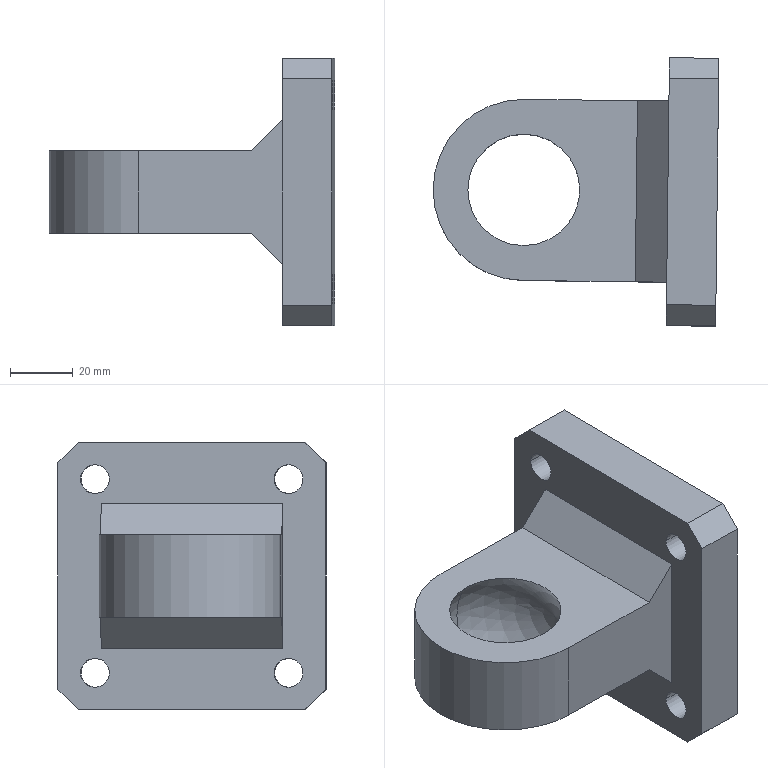Part | STEP file | Multi-stage electric cylinder rear end | 1 solid | 31 faces | box 90.745 x 85.184 x 85 mm | volume 182065 mm3 | plane 16 | cylinder 13 | sphere 2 | commonest cylinder face diameters 9.154 x8 57.538 x3 41.153 x2
STEP:
#1=CARTESIAN_POINT('',(-3126.978,-89.796,4204.56));
#2=VERTEX_POINT('',#1);
#3=CARTESIAN_POINT('',(-3136.48,-107.138,4204.56));
#4=VERTEX_POINT('',#3);
#5=CARTESIAN_POINT('',(-3115.903,-107.138,4204.56));
#6=DIRECTION('',(0.,0.,1.));
#7=DIRECTION('',(1.,0.,0.));
#8=AXIS2_PLACEMENT_3D('',#5,#6,#7);
#9=CIRCLE('',#8,20.576);
#10=EDGE_CURVE('',#2,#4,#9,.T.);
#11=ORIENTED_EDGE('',*,*,#10,.T.);
#12=CARTESIAN_POINT('',(-3136.48,-107.138,4188.867));
#13=VERTEX_POINT('',#12);
#14=CARTESIAN_POINT('',(-3136.48,-107.138,4275.262));
#15=DIRECTION('',(0.,0.,-1.));
#16=VECTOR('',#15,1000.);
#17=LINE('',#14,#16);
#18=EDGE_CURVE('',#4,#13,#17,.T.);
#19=ORIENTED_EDGE('',*,*,#18,.T.);
#20=CARTESIAN_POINT('',(-3126.978,-89.796,4188.867));
#21=VERTEX_POINT('',#20);
#22=CARTESIAN_POINT('',(-3115.903,-107.138,4188.867));
#23=DIRECTION('',(0.,0.,1.));
#24=DIRECTION('',(1.,0.,0.));
#25=AXIS2_PLACEMENT_3D('',#22,#23,#24);
#26=CIRCLE('',#25,20.576);
#27=EDGE_CURVE('',#21,#13,#26,.T.);
#28=ORIENTED_EDGE('',*,*,#27,.F.);
#29=CARTESIAN_POINT('',(-3126.978,-89.796,4275.262));
#30=DIRECTION('',(0.,0.,-1.));
#31=VECTOR('',#30,1000.);
#32=LINE('',#29,#31);
#33=EDGE_CURVE('',#2,#21,#32,.T.);
#34=ORIENTED_EDGE('',*,*,#33,.F.);
#35=EDGE_LOOP('',(#11,#19,#28,#34));
#36=FACE_OUTER_BOUND('',#35,.T.);
#37=CARTESIAN_POINT('',(-3115.903,-107.138,4275.262));
#38=DIRECTION('',(0.,0.,-1.));
#39=DIRECTION('',(-1.,0.,0.));
#40=AXIS2_PLACEMENT_3D('',#37,#38,#39);
#41=CYLINDRICAL_SURFACE('',#40,20.576);
#42=ADVANCED_FACE('',(#36),#41,.F.);
#43=CARTESIAN_POINT('',(-3070.562,-142.998,4165.983));
#44=VERTEX_POINT('',#43);
#45=CARTESIAN_POINT('',(-3070.451,-133.845,4165.983));
#46=VERTEX_POINT('',#45);
#47=CARTESIAN_POINT('',(-3070.507,-138.421,4165.983));
#48=DIRECTION('',(0.9999,-0.01213,0.));
#49=DIRECTION('',(0.01213,0.9999,0.));
#50=AXIS2_PLACEMENT_3D('',#47,#48,#49);
#51=CIRCLE('',#50,4.577);
#52=EDGE_CURVE('',#44,#46,#51,.T.);
#53=ORIENTED_EDGE('',*,*,#52,.F.);
#54=CARTESIAN_POINT('',(-3054.871,-143.188,4165.983));
#55=VERTEX_POINT('',#54);
#56=CARTESIAN_POINT('',(-3054.871,-143.188,4165.983));
#57=DIRECTION('',(0.9999,-0.01213,0.));
#58=VECTOR('',#57,1000.);
#59=LINE('',#56,#58);
#60=EDGE_CURVE('',#44,#55,#59,.T.);
#61=ORIENTED_EDGE('',*,*,#60,.T.);
#62=CARTESIAN_POINT('',(-3054.76,-134.035,4165.983));
#63=VERTEX_POINT('',#62);
#64=CARTESIAN_POINT('',(-3054.816,-138.612,4165.983));
#65=DIRECTION('',(0.9999,-0.01213,0.));
#66=DIRECTION('',(0.01213,0.9999,0.));
#67=AXIS2_PLACEMENT_3D('',#64,#65,#66);
#68=CIRCLE('',#67,4.577);
#69=EDGE_CURVE('',#55,#63,#68,.T.);
#70=ORIENTED_EDGE('',*,*,#69,.T.);
#71=CARTESIAN_POINT('',(-3054.76,-134.035,4165.983));
#72=DIRECTION('',(0.9999,-0.01213,0.));
#73=VECTOR('',#72,1000.);
#74=LINE('',#71,#73);
#75=EDGE_CURVE('',#46,#63,#74,.T.);
#76=ORIENTED_EDGE('',*,*,#75,.F.);
#77=EDGE_LOOP('',(#53,#61,#70,#76));
#78=FACE_OUTER_BOUND('',#77,.T.);
#79=CARTESIAN_POINT('',(-3054.816,-138.612,4165.983));
#80=DIRECTION('',(0.9999,-0.01213,0.));
#81=DIRECTION('',(0.01213,0.9999,0.));
#82=AXIS2_PLACEMENT_3D('',#79,#80,#81);
#83=CYLINDRICAL_SURFACE('',#82,4.577);
#84=ADVANCED_FACE('',(#78),#83,.F.);
#85=CARTESIAN_POINT('',(-3069.817,-81.541,4165.983));
#86=VERTEX_POINT('',#85);
#87=CARTESIAN_POINT('',(-3069.706,-72.388,4165.983));
#88=VERTEX_POINT('',#87);
#89=CARTESIAN_POINT('',(-3069.761,-76.964,4165.983));
#90=DIRECTION('',(0.9999,-0.01213,0.));
#91=DIRECTION('',(0.01213,0.9999,0.));
#92=AXIS2_PLACEMENT_3D('',#89,#90,#91);
#93=CIRCLE('',#92,4.577);
#94=EDGE_CURVE('',#86,#88,#93,.T.);
#95=ORIENTED_EDGE('',*,*,#94,.F.);
#96=CARTESIAN_POINT('',(-3054.126,-81.731,4165.983));
#97=VERTEX_POINT('',#96);
#98=CARTESIAN_POINT('',(-3054.126,-81.731,4165.983));
#99=DIRECTION('',(0.9999,-0.01213,0.));
#100=VECTOR('',#99,1000.);
#101=LINE('',#98,#100);
#102=EDGE_CURVE('',#86,#97,#101,.T.);
#103=ORIENTED_EDGE('',*,*,#102,.T.);
#104=CARTESIAN_POINT('',(-3054.015,-72.578,4165.983));
#105=VERTEX_POINT('',#104);
#106=CARTESIAN_POINT('',(-3054.07,-77.155,4165.983));
#107=DIRECTION('',(0.9999,-0.01213,0.));
#108=DIRECTION('',(0.01213,0.9999,0.));
#109=AXIS2_PLACEMENT_3D('',#106,#107,#108);
#110=CIRCLE('',#109,4.577);
#111=EDGE_CURVE('',#97,#105,#110,.T.);
#112=ORIENTED_EDGE('',*,*,#111,.T.);
#113=CARTESIAN_POINT('',(-3054.015,-72.578,4165.983));
#114=DIRECTION('',(0.9999,-0.01213,0.));
#115=VECTOR('',#114,1000.);
#116=LINE('',#113,#115);
#117=EDGE_CURVE('',#88,#105,#116,.T.);
#118=ORIENTED_EDGE('',*,*,#117,.F.);
#119=EDGE_LOOP('',(#95,#103,#112,#118));
#120=FACE_OUTER_BOUND('',#119,.T.);
#121=CARTESIAN_POINT('',(-3054.07,-77.155,4165.983));
#122=DIRECTION('',(0.9999,-0.01213,0.));
#123=DIRECTION('',(0.01213,0.9999,0.));
#124=AXIS2_PLACEMENT_3D('',#121,#122,#123);
#125=CYLINDRICAL_SURFACE('',#124,4.577);
#126=ADVANCED_FACE('',(#120),#125,.F.);
#127=CARTESIAN_POINT('',(-3069.817,-81.541,4227.444));
#128=VERTEX_POINT('',#127);
#129=CARTESIAN_POINT('',(-3069.706,-72.388,4227.444));
#130=VERTEX_POINT('',#129);
#131=CARTESIAN_POINT('',(-3069.761,-76.964,4227.444));
#132=DIRECTION('',(0.9999,-0.01213,0.));
#133=DIRECTION('',(0.01213,0.9999,0.));
#134=AXIS2_PLACEMENT_3D('',#131,#132,#133);
#135=CIRCLE('',#134,4.577);
#136=EDGE_CURVE('',#128,#130,#135,.T.);
#137=ORIENTED_EDGE('',*,*,#136,.F.);
#138=CARTESIAN_POINT('',(-3054.126,-81.731,4227.444));
#139=VERTEX_POINT('',#138);
#140=CARTESIAN_POINT('',(-3054.126,-81.731,4227.444));
#141=DIRECTION('',(0.9999,-0.01213,0.));
#142=VECTOR('',#141,1000.);
#143=LINE('',#140,#142);
#144=EDGE_CURVE('',#128,#139,#143,.T.);
#145=ORIENTED_EDGE('',*,*,#144,.T.);
#146=CARTESIAN_POINT('',(-3054.015,-72.578,4227.444));
#147=VERTEX_POINT('',#146);
#148=CARTESIAN_POINT('',(-3054.07,-77.155,4227.444));
#149=DIRECTION('',(0.9999,-0.01213,0.));
#150=DIRECTION('',(0.01213,0.9999,0.));
#151=AXIS2_PLACEMENT_3D('',#148,#149,#150);
#152=CIRCLE('',#151,4.577);
#153=EDGE_CURVE('',#139,#147,#152,.T.);
#154=ORIENTED_EDGE('',*,*,#153,.T.);
#155=CARTESIAN_POINT('',(-3054.015,-72.578,4227.444));
#156=DIRECTION('',(0.9999,-0.01213,0.));
#157=VECTOR('',#156,1000.);
#158=LINE('',#155,#157);
#159=EDGE_CURVE('',#130,#147,#158,.T.);
#160=ORIENTED_EDGE('',*,*,#159,.F.);
#161=EDGE_LOOP('',(#137,#145,#154,#160));
#162=FACE_OUTER_BOUND('',#161,.T.);
#163=CARTESIAN_POINT('',(-3054.07,-77.155,4227.444));
#164=DIRECTION('',(0.9999,-0.01213,0.));
#165=DIRECTION('',(0.01213,0.9999,0.));
#166=AXIS2_PLACEMENT_3D('',#163,#164,#165);
#167=CYLINDRICAL_SURFACE('',#166,4.577);
#168=ADVANCED_FACE('',(#162),#167,.F.);
#169=CARTESIAN_POINT('',(-3070.562,-142.998,4227.444));
#170=VERTEX_POINT('',#169);
#171=CARTESIAN_POINT('',(-3070.451,-133.845,4227.444));
#172=VERTEX_POINT('',#171);
#173=CARTESIAN_POINT('',(-3070.507,-138.421,4227.444));
#174=DIRECTION('',(0.9999,-0.01213,0.));
#175=DIRECTION('',(0.01213,0.9999,0.));
#176=AXIS2_PLACEMENT_3D('',#173,#174,#175);
#177=CIRCLE('',#176,4.577);
#178=EDGE_CURVE('',#170,#172,#177,.T.);
#179=ORIENTED_EDGE('',*,*,#178,.F.);
#180=CARTESIAN_POINT('',(-3054.871,-143.188,4227.444));
#181=VERTEX_POINT('',#180);
#182=CARTESIAN_POINT('',(-3054.871,-143.188,4227.444));
#183=DIRECTION('',(0.9999,-0.01213,0.));
#184=VECTOR('',#183,1000.);
#185=LINE('',#182,#184);
#186=EDGE_CURVE('',#170,#181,#185,.T.);
#187=ORIENTED_EDGE('',*,*,#186,.T.);
#188=CARTESIAN_POINT('',(-3054.76,-134.035,4227.444));
#189=VERTEX_POINT('',#188);
#190=CARTESIAN_POINT('',(-3054.816,-138.612,4227.444));
#191=DIRECTION('',(0.9999,-0.01213,0.));
#192=DIRECTION('',(0.01213,0.9999,0.));
#193=AXIS2_PLACEMENT_3D('',#190,#191,#192);
#194=CIRCLE('',#193,4.577);
#195=EDGE_CURVE('',#181,#189,#194,.T.);
#196=ORIENTED_EDGE('',*,*,#195,.T.);
#197=CARTESIAN_POINT('',(-3054.76,-134.035,4227.444));
#198=DIRECTION('',(0.9999,-0.01213,0.));
#199=VECTOR('',#198,1000.);
#200=LINE('',#197,#199);
#201=EDGE_CURVE('',#172,#189,#200,.T.);
#202=ORIENTED_EDGE('',*,*,#201,.F.);
#203=EDGE_LOOP('',(#179,#187,#196,#202));
#204=FACE_OUTER_BOUND('',#203,.T.);
#205=CARTESIAN_POINT('',(-3054.816,-138.612,4227.444));
#206=DIRECTION('',(0.9999,-0.01213,0.));
#207=DIRECTION('',(0.01213,0.9999,0.));
#208=AXIS2_PLACEMENT_3D('',#205,#206,#207);
#209=CYLINDRICAL_SURFACE('',#208,4.577);
#210=ADVANCED_FACE('',(#204),#209,.F.);
#211=ORIENTED_EDGE('',*,*,#10,.F.);
#212=CARTESIAN_POINT('',(-3126.978,-89.796,4188.867));
#213=CARTESIAN_POINT('',(-3126.634,-89.346,4189.376));
#214=CARTESIAN_POINT('',(-3126.301,-88.939,4189.916));
#215=CARTESIAN_POINT('',(-3125.834,-88.393,4190.788));
#216=CARTESIAN_POINT('',(-3125.684,-88.223,4191.088));
#217=CARTESIAN_POINT('',(-3125.399,-87.905,4191.712));
#218=CARTESIAN_POINT('',(-3125.263,-87.757,4192.037));
#219=CARTESIAN_POINT('',(-3124.889,-87.357,4193.037));
#220=CARTESIAN_POINT('',(-3124.686,-87.15,4193.733));
#221=CARTESIAN_POINT('',(-3124.473,-86.936,4194.83));
#222=CARTESIAN_POINT('',(-3124.418,-86.882,4195.207));
#223=CARTESIAN_POINT('',(-3124.345,-86.809,4195.957));
#224=CARTESIAN_POINT('',(-3124.327,-86.791,4196.332));
#225=CARTESIAN_POINT('',(-3124.327,-86.791,4197.083));
#226=CARTESIAN_POINT('',(-3124.345,-86.809,4197.459));
#227=CARTESIAN_POINT('',(-3124.417,-86.881,4198.213));
#228=CARTESIAN_POINT('',(-3124.472,-86.935,4198.589));
#229=CARTESIAN_POINT('',(-3124.613,-87.077,4199.319));
#230=CARTESIAN_POINT('',(-3124.699,-87.164,4199.676));
#231=CARTESIAN_POINT('',(-3124.899,-87.37,4200.377));
#232=CARTESIAN_POINT('',(-3125.013,-87.49,4200.722));
#233=CARTESIAN_POINT('',(-3125.387,-87.89,4201.723));
#234=CARTESIAN_POINT('',(-3125.675,-88.208,4202.342));
#235=CARTESIAN_POINT('',(-3126.297,-88.935,4203.505));
#236=CARTESIAN_POINT('',(-3126.634,-89.346,4204.051));
#237=CARTESIAN_POINT('',(-3126.978,-89.796,4204.56));
#238=B_SPLINE_CURVE_WITH_KNOTS('',3,(#212,#213,#214,#215,#216,#217,#218,#219,#220,#221,#222,#223,#224,#225,#226,#227,#228,#229,#230,#231,#232,#233,#234,#235,#236,#237),.UNSPECIFIED.,.F.,.F.,(4,2,2,2,2,2,2,2,2,2,2,2,4),(0.000000387,0.002258,0.003387,0.004516,0.006773,0.007902,0.009031,0.01016,0.01129,0.01242,0.01355,0.0158,0.01806),.UNSPECIFIED.);
#239=EDGE_CURVE('',#21,#2,#238,.T.);
#240=ORIENTED_EDGE('',*,*,#239,.F.);
#241=ORIENTED_EDGE('',*,*,#27,.T.);
#242=CARTESIAN_POINT('',(-3127.395,-124.206,4188.867));
#243=VERTEX_POINT('',#242);
#244=CARTESIAN_POINT('',(-3115.903,-107.138,4188.867));
#245=DIRECTION('',(0.,0.,1.));
#246=DIRECTION('',(1.,0.,0.));
#247=AXIS2_PLACEMENT_3D('',#244,#245,#246);
#248=CIRCLE('',#247,20.576);
#249=EDGE_CURVE('',#13,#243,#248,.T.);
#250=ORIENTED_EDGE('',*,*,#249,.T.);
#251=CARTESIAN_POINT('',(-3127.395,-124.206,4204.56));
#252=VERTEX_POINT('',#251);
#253=CARTESIAN_POINT('',(-3127.395,-124.206,4204.56));
#254=CARTESIAN_POINT('',(-3127.062,-124.664,4204.052));
#255=CARTESIAN_POINT('',(-3126.739,-125.08,4203.511));
#256=CARTESIAN_POINT('',(-3126.286,-125.636,4202.639));
#257=CARTESIAN_POINT('',(-3126.14,-125.81,4202.339));
#258=CARTESIAN_POINT('',(-3125.862,-126.135,4201.715));
#259=CARTESIAN_POINT('',(-3125.73,-126.286,4201.39));
#260=CARTESIAN_POINT('',(-3125.366,-126.695,4200.39));
#261=CARTESIAN_POINT('',(-3125.168,-126.907,4199.694));
#262=CARTESIAN_POINT('',(-3124.961,-127.126,4198.597));
#263=CARTESIAN_POINT('',(-3124.907,-127.182,4198.22));
#264=CARTESIAN_POINT('',(-3124.836,-127.256,4197.471));
#265=CARTESIAN_POINT('',(-3124.818,-127.274,4197.095));
#266=CARTESIAN_POINT('',(-3124.817,-127.275,4196.344));
#267=CARTESIAN_POINT('',(-3124.835,-127.257,4195.968));
#268=CARTESIAN_POINT('',(-3124.906,-127.183,4195.214));
#269=CARTESIAN_POINT('',(-3124.96,-127.127,4194.839));
#270=CARTESIAN_POINT('',(-3125.097,-126.982,4194.108));
#271=CARTESIAN_POINT('',(-3125.181,-126.893,4193.751));
#272=CARTESIAN_POINT('',(-3125.375,-126.682,4193.05));
#273=CARTESIAN_POINT('',(-3125.487,-126.559,4192.705));
#274=CARTESIAN_POINT('',(-3125.851,-126.151,4191.705));
#275=CARTESIAN_POINT('',(-3126.131,-125.826,4191.086));
#276=CARTESIAN_POINT('',(-3126.736,-125.084,4189.922));
#277=CARTESIAN_POINT('',(-3127.062,-124.664,4189.376));
#278=CARTESIAN_POINT('',(-3127.395,-124.206,4188.867));
#279=B_SPLINE_CURVE_WITH_KNOTS('',3,(#253,#254,#255,#256,#257,#258,#259,#260,#261,#262,#263,#264,#265,#266,#267,#268,#269,#270,#271,#272,#273,#274,#275,#276,#277,#278),.UNSPECIFIED.,.F.,.F.,(4,2,2,2,2,2,2,2,2,2,2,2,4),(0.000000387,0.002258,0.003387,0.004516,0.006773,0.007902,0.009031,0.01016,0.01129,0.01242,0.01355,0.0158,0.01806),.UNSPECIFIED.);
#280=EDGE_CURVE('',#252,#243,#279,.T.);
#281=ORIENTED_EDGE('',*,*,#280,.F.);
#282=CARTESIAN_POINT('',(-3115.903,-107.138,4204.56));
#283=DIRECTION('',(0.,0.,1.));
#284=DIRECTION('',(1.,0.,0.));
#285=AXIS2_PLACEMENT_3D('',#282,#283,#284);
#286=CIRCLE('',#285,20.576);
#287=EDGE_CURVE('',#4,#252,#286,.T.);
#288=ORIENTED_EDGE('',*,*,#287,.F.);
#289=EDGE_LOOP('',(#211,#240,#241,#250,#281,#288));
#290=FACE_BOUND('',#289,.T.);
#291=CARTESIAN_POINT('',(-3115.688,-89.421,4209.79));
#292=VERTEX_POINT('',#291);
#293=CARTESIAN_POINT('',(-3116.118,-124.855,4209.79));
#294=VERTEX_POINT('',#293);
#295=CARTESIAN_POINT('',(-3115.903,-107.138,4209.79));
#296=DIRECTION('',(0.,0.,1.));
#297=DIRECTION('',(-1.,0.,0.));
#298=AXIS2_PLACEMENT_3D('',#295,#296,#297);
#299=CIRCLE('',#298,17.718);
#300=EDGE_CURVE('',#292,#294,#299,.T.);
#301=ORIENTED_EDGE('',*,*,#300,.T.);
#302=CARTESIAN_POINT('',(-3116.118,-124.855,4183.637));
#303=VERTEX_POINT('',#302);
#304=CARTESIAN_POINT('',(-3115.903,-107.138,4196.714));
#305=DIRECTION('',(0.9999,-0.01213,0.));
#306=DIRECTION('',(0.01213,0.9999,0.));
#307=AXIS2_PLACEMENT_3D('',#304,#305,#306);
#308=CIRCLE('',#307,22.022);
#309=EDGE_CURVE('',#294,#303,#308,.T.);
#310=ORIENTED_EDGE('',*,*,#309,.T.);
#311=CARTESIAN_POINT('',(-3115.688,-89.421,4183.637));
#312=VERTEX_POINT('',#311);
#313=CARTESIAN_POINT('',(-3115.903,-107.138,4183.637));
#314=DIRECTION('',(0.,0.,1.));
#315=DIRECTION('',(-1.,0.,0.));
#316=AXIS2_PLACEMENT_3D('',#313,#314,#315);
#317=CIRCLE('',#316,17.718);
#318=EDGE_CURVE('',#312,#303,#317,.T.);
#319=ORIENTED_EDGE('',*,*,#318,.F.);
#320=CARTESIAN_POINT('',(-3115.903,-107.138,4196.714));
#321=DIRECTION('',(-0.9999,0.01213,0.));
#322=DIRECTION('',(-0.01213,-0.9999,0.));
#323=AXIS2_PLACEMENT_3D('',#320,#321,#322);
#324=CIRCLE('',#323,22.022);
#325=EDGE_CURVE('',#292,#312,#324,.T.);
#326=ORIENTED_EDGE('',*,*,#325,.F.);
#327=EDGE_LOOP('',(#301,#310,#319,#326));
#328=FACE_OUTER_BOUND('',#327,.T.);
#329=CARTESIAN_POINT('',(-3115.903,-107.138,4196.714));
#330=DIRECTION('',(0.9999,-0.01213,0.));
#331=DIRECTION('',(0.01213,0.9999,0.));
#332=AXIS2_PLACEMENT_3D('',#329,#330,#331);
#333=SPHERICAL_SURFACE('',#332,22.022);
#334=ADVANCED_FACE('',(#290,#328),#333,.F.);
#335=CARTESIAN_POINT('',(-3115.554,-78.371,4183.637));
#336=VERTEX_POINT('',#335);
#337=CARTESIAN_POINT('',(-3079.785,-78.805,4183.637));
#338=VERTEX_POINT('',#337);
#339=CARTESIAN_POINT('',(-3174.393,-77.657,4183.637));
#340=DIRECTION('',(0.9999,-0.01213,0.));
#341=VECTOR('',#340,1000.);
#342=LINE('',#339,#341);
#343=EDGE_CURVE('',#336,#338,#342,.T.);
#344=ORIENTED_EDGE('',*,*,#343,.F.);
#345=CARTESIAN_POINT('',(-3115.554,-78.371,4209.79));
#346=VERTEX_POINT('',#345);
#347=CARTESIAN_POINT('',(-3115.554,-78.371,4204.56));
#348=DIRECTION('',(0.,0.,1.));
#349=VECTOR('',#348,1000.);
#350=LINE('',#347,#349);
#351=EDGE_CURVE('',#336,#346,#350,.T.);
#352=ORIENTED_EDGE('',*,*,#351,.T.);
#353=CARTESIAN_POINT('',(-3079.785,-78.805,4209.79));
#354=VERTEX_POINT('',#353);
#355=CARTESIAN_POINT('',(-3174.393,-77.657,4209.79));
#356=DIRECTION('',(0.9999,-0.01213,0.));
#357=VECTOR('',#356,1000.);
#358=LINE('',#355,#357);
#359=EDGE_CURVE('',#346,#354,#358,.T.);
#360=ORIENTED_EDGE('',*,*,#359,.T.);
#361=CARTESIAN_POINT('',(-3069.785,-78.926,4219.79));
#362=VERTEX_POINT('',#361);
#363=CARTESIAN_POINT('',(-3079.785,-78.805,4209.79));
#364=DIRECTION('',(0.7071,-0.008574,0.7071));
#365=VECTOR('',#364,1000.);
#366=LINE('',#363,#365);
#367=EDGE_CURVE('',#354,#362,#366,.T.);
#368=ORIENTED_EDGE('',*,*,#367,.T.);
#369=CARTESIAN_POINT('',(-3069.785,-78.926,4173.637));
#370=VERTEX_POINT('',#369);
#371=CARTESIAN_POINT('',(-3069.785,-78.926,4204.56));
#372=DIRECTION('',(0.,0.,1.));
#373=VECTOR('',#372,1000.);
#374=LINE('',#371,#373);
#375=EDGE_CURVE('',#370,#362,#374,.T.);
#376=ORIENTED_EDGE('',*,*,#375,.F.);
#377=CARTESIAN_POINT('',(-3069.785,-78.926,4173.637));
#378=DIRECTION('',(-0.7071,0.008574,0.7071));
#379=VECTOR('',#378,1000.);
#380=LINE('',#377,#379);
#381=EDGE_CURVE('',#370,#338,#380,.T.);
#382=ORIENTED_EDGE('',*,*,#381,.T.);
#383=EDGE_LOOP('',(#344,#352,#360,#368,#376,#382));
#384=FACE_OUTER_BOUND('',#383,.T.);
#385=CARTESIAN_POINT('',(-3069.785,-78.926,4204.56));
#386=DIRECTION('',(0.01213,0.9999,0.));
#387=DIRECTION('',(-0.9999,0.01213,0.));
#388=AXIS2_PLACEMENT_3D('',#385,#386,#387);
#389=PLANE('',#388);
#390=ADVANCED_FACE('',(#384),#389,.T.);
#391=CARTESIAN_POINT('',(-3116.252,-135.905,4183.637));
#392=VERTEX_POINT('',#391);
#393=CARTESIAN_POINT('',(-3116.252,-135.905,4209.79));
#394=VERTEX_POINT('',#393);
#395=CARTESIAN_POINT('',(-3116.252,-135.905,4204.56));
#396=DIRECTION('',(0.,0.,1.));
#397=VECTOR('',#396,1000.);
#398=LINE('',#395,#397);
#399=EDGE_CURVE('',#392,#394,#398,.T.);
#400=ORIENTED_EDGE('',*,*,#399,.F.);
#401=CARTESIAN_POINT('',(-3080.482,-136.339,4183.637));
#402=VERTEX_POINT('',#401);
#403=CARTESIAN_POINT('',(-3175.091,-135.192,4183.637));
#404=DIRECTION('',(0.9999,-0.01213,0.));
#405=VECTOR('',#404,1000.);
#406=LINE('',#403,#405);
#407=EDGE_CURVE('',#392,#402,#406,.T.);
#408=ORIENTED_EDGE('',*,*,#407,.T.);
#409=CARTESIAN_POINT('',(-3070.483,-136.46,4173.637));
#410=VERTEX_POINT('',#409);
#411=CARTESIAN_POINT('',(-3070.483,-136.46,4173.637));
#412=DIRECTION('',(0.7071,-0.008574,-0.7071));
#413=VECTOR('',#412,1000.);
#414=LINE('',#411,#413);
#415=EDGE_CURVE('',#402,#410,#414,.T.);
#416=ORIENTED_EDGE('',*,*,#415,.T.);
#417=CARTESIAN_POINT('',(-3070.483,-136.46,4219.79));
#418=VERTEX_POINT('',#417);
#419=CARTESIAN_POINT('',(-3070.483,-136.46,4204.56));
#420=DIRECTION('',(0.,0.,1.));
#421=VECTOR('',#420,1000.);
#422=LINE('',#419,#421);
#423=EDGE_CURVE('',#410,#418,#422,.T.);
#424=ORIENTED_EDGE('',*,*,#423,.T.);
#425=CARTESIAN_POINT('',(-3080.482,-136.339,4209.79));
#426=VERTEX_POINT('',#425);
#427=CARTESIAN_POINT('',(-3080.482,-136.339,4209.79));
#428=DIRECTION('',(-0.7071,0.008574,-0.7071));
#429=VECTOR('',#428,1000.);
#430=LINE('',#427,#429);
#431=EDGE_CURVE('',#418,#426,#430,.T.);
#432=ORIENTED_EDGE('',*,*,#431,.T.);
#433=CARTESIAN_POINT('',(-3175.091,-135.192,4209.79));
#434=DIRECTION('',(0.9999,-0.01213,0.));
#435=VECTOR('',#434,1000.);
#436=LINE('',#433,#435);
#437=EDGE_CURVE('',#394,#426,#436,.T.);
#438=ORIENTED_EDGE('',*,*,#437,.F.);
#439=EDGE_LOOP('',(#400,#408,#416,#424,#432,#438));
#440=FACE_OUTER_BOUND('',#439,.T.);
#441=CARTESIAN_POINT('',(-3116.252,-135.905,4204.56));
#442=DIRECTION('',(-0.01213,-0.9999,0.));
#443=DIRECTION('',(0.9999,-0.01213,0.));
#444=AXIS2_PLACEMENT_3D('',#441,#442,#443);
#445=PLANE('',#444);
#446=ADVANCED_FACE('',(#440),#445,.T.);
#447=ORIENTED_EDGE('',*,*,#309,.F.);
#448=CARTESIAN_POINT('',(-3115.903,-107.138,4209.79));
#449=DIRECTION('',(0.,0.,1.));
#450=DIRECTION('',(-1.,0.,0.));
#451=AXIS2_PLACEMENT_3D('',#448,#449,#450);
#452=CIRCLE('',#451,17.718);
#453=EDGE_CURVE('',#294,#292,#452,.T.);
#454=ORIENTED_EDGE('',*,*,#453,.T.);
#455=ORIENTED_EDGE('',*,*,#325,.T.);
#456=CARTESIAN_POINT('',(-3115.903,-107.138,4183.637));
#457=DIRECTION('',(0.,0.,1.));
#458=DIRECTION('',(-1.,0.,0.));
#459=AXIS2_PLACEMENT_3D('',#456,#457,#458);
#460=CIRCLE('',#459,17.718);
#461=EDGE_CURVE('',#303,#312,#460,.T.);
#462=ORIENTED_EDGE('',*,*,#461,.F.);
#463=EDGE_LOOP('',(#447,#454,#455,#462));
#464=FACE_OUTER_BOUND('',#463,.T.);
#465=CARTESIAN_POINT('',(-3115.903,-107.138,4196.714));
#466=DIRECTION('',(0.9999,-0.01213,0.));
#467=DIRECTION('',(0.01213,0.9999,0.));
#468=AXIS2_PLACEMENT_3D('',#465,#466,#467);
#469=SPHERICAL_SURFACE('',#468,22.022);
#470=ADVANCED_FACE('',(#464),#469,.F.);
#471=CARTESIAN_POINT('',(-3067.836,81.794,4173.637));
#472=DIRECTION('',(0.01213,0.9999,0.));
#473=VECTOR('',#472,1000.);
#474=LINE('',#471,#473);
#475=EDGE_CURVE('',#410,#370,#474,.T.);
#476=ORIENTED_EDGE('',*,*,#475,.T.);
#477=ORIENTED_EDGE('',*,*,#375,.T.);
#478=CARTESIAN_POINT('',(-3070.483,-136.46,4219.79));
#479=DIRECTION('',(-0.01213,-0.9999,0.));
#480=VECTOR('',#479,1000.);
#481=LINE('',#478,#480);
#482=EDGE_CURVE('',#362,#418,#481,.T.);
#483=ORIENTED_EDGE('',*,*,#482,.T.);
#484=ORIENTED_EDGE('',*,*,#423,.F.);
#485=EDGE_LOOP('',(#476,#477,#483,#484));
#486=FACE_BOUND('',#485,.T.);
#487=CARTESIAN_POINT('',(-3070.649,-150.19,4232.675));
#488=VERTEX_POINT('',#487);
#489=CARTESIAN_POINT('',(-3070.649,-150.19,4160.752));
#490=VERTEX_POINT('',#489);
#491=CARTESIAN_POINT('',(-3070.649,-150.19,4239.214));
#492=DIRECTION('',(0.,0.,-1.));
#493=VECTOR('',#492,1000.);
#494=LINE('',#491,#493);
#495=EDGE_CURVE('',#488,#490,#494,.T.);
#496=ORIENTED_EDGE('',*,*,#495,.F.);
#497=CARTESIAN_POINT('',(-3070.57,-143.652,4239.214));
#498=VERTEX_POINT('',#497);
#499=CARTESIAN_POINT('',(-3070.57,-143.652,4239.214));
#500=DIRECTION('',(0.008574,0.7071,0.7071));
#501=VECTOR('',#500,1000.);
#502=LINE('',#499,#501);
#503=EDGE_CURVE('',#488,#498,#502,.T.);
#504=ORIENTED_EDGE('',*,*,#503,.T.);
#505=CARTESIAN_POINT('',(-3069.698,-71.734,4239.214));
#506=VERTEX_POINT('',#505);
#507=CARTESIAN_POINT('',(-3069.619,-65.196,4239.214));
#508=DIRECTION('',(-0.01213,-0.9999,0.));
#509=VECTOR('',#508,1000.);
#510=LINE('',#507,#509);
#511=EDGE_CURVE('',#506,#498,#510,.T.);
#512=ORIENTED_EDGE('',*,*,#511,.F.);
#513=CARTESIAN_POINT('',(-3069.619,-65.196,4232.675));
#514=VERTEX_POINT('',#513);
#515=CARTESIAN_POINT('',(-3069.619,-65.196,4232.675));
#516=DIRECTION('',(0.008574,0.7071,-0.7071));
#517=VECTOR('',#516,1000.);
#518=LINE('',#515,#517);
#519=EDGE_CURVE('',#506,#514,#518,.T.);
#520=ORIENTED_EDGE('',*,*,#519,.T.);
#521=CARTESIAN_POINT('',(-3069.619,-65.196,4160.752));
#522=VERTEX_POINT('',#521);
#523=CARTESIAN_POINT('',(-3069.619,-65.196,4154.214));
#524=DIRECTION('',(0.,0.,1.));
#525=VECTOR('',#524,1000.);
#526=LINE('',#523,#525);
#527=EDGE_CURVE('',#522,#514,#526,.T.);
#528=ORIENTED_EDGE('',*,*,#527,.F.);
#529=CARTESIAN_POINT('',(-3069.698,-71.734,4154.214));
#530=VERTEX_POINT('',#529);
#531=CARTESIAN_POINT('',(-3069.698,-71.734,4154.214));
#532=DIRECTION('',(-0.008574,-0.7071,-0.7071));
#533=VECTOR('',#532,1000.);
#534=LINE('',#531,#533);
#535=EDGE_CURVE('',#522,#530,#534,.T.);
#536=ORIENTED_EDGE('',*,*,#535,.T.);
#537=CARTESIAN_POINT('',(-3070.57,-143.652,4154.214));
#538=VERTEX_POINT('',#537);
#539=CARTESIAN_POINT('',(-3070.649,-150.19,4154.214));
#540=DIRECTION('',(0.01213,0.9999,0.));
#541=VECTOR('',#540,1000.);
#542=LINE('',#539,#541);
#543=EDGE_CURVE('',#538,#530,#542,.T.);
#544=ORIENTED_EDGE('',*,*,#543,.F.);
#545=CARTESIAN_POINT('',(-3070.649,-150.19,4160.752));
#546=DIRECTION('',(-0.008574,-0.7071,0.7071));
#547=VECTOR('',#546,1000.);
#548=LINE('',#545,#547);
#549=EDGE_CURVE('',#538,#490,#548,.T.);
#550=ORIENTED_EDGE('',*,*,#549,.T.);
#551=EDGE_LOOP('',(#496,#504,#512,#520,#528,#536,#544,#550));
#552=FACE_OUTER_BOUND('',#551,.T.);
#553=CARTESIAN_POINT('',(-3070.507,-138.421,4227.444));
#554=DIRECTION('',(0.9999,-0.01213,0.));
#555=DIRECTION('',(0.01213,0.9999,0.));
#556=AXIS2_PLACEMENT_3D('',#553,#554,#555);
#557=CIRCLE('',#556,4.577);
#558=EDGE_CURVE('',#172,#170,#557,.T.);
#559=ORIENTED_EDGE('',*,*,#558,.T.);
#560=ORIENTED_EDGE('',*,*,#178,.T.);
#561=EDGE_LOOP('',(#559,#560));
#562=FACE_BOUND('',#561,.T.);
#563=CARTESIAN_POINT('',(-3069.761,-76.964,4227.444));
#564=DIRECTION('',(0.9999,-0.01213,0.));
#565=DIRECTION('',(0.01213,0.9999,0.));
#566=AXIS2_PLACEMENT_3D('',#563,#564,#565);
#567=CIRCLE('',#566,4.577);
#568=EDGE_CURVE('',#130,#128,#567,.T.);
#569=ORIENTED_EDGE('',*,*,#568,.T.);
#570=ORIENTED_EDGE('',*,*,#136,.T.);
#571=EDGE_LOOP('',(#569,#570));
#572=FACE_BOUND('',#571,.T.);
#573=CARTESIAN_POINT('',(-3069.761,-76.964,4165.983));
#574=DIRECTION('',(0.9999,-0.01213,0.));
#575=DIRECTION('',(0.01213,0.9999,0.));
#576=AXIS2_PLACEMENT_3D('',#573,#574,#575);
#577=CIRCLE('',#576,4.577);
#578=EDGE_CURVE('',#88,#86,#577,.T.);
#579=ORIENTED_EDGE('',*,*,#578,.T.);
#580=ORIENTED_EDGE('',*,*,#94,.T.);
#581=EDGE_LOOP('',(#579,#580));
#582=FACE_BOUND('',#581,.T.);
#583=CARTESIAN_POINT('',(-3070.507,-138.421,4165.983));
#584=DIRECTION('',(0.9999,-0.01213,0.));
#585=DIRECTION('',(0.01213,0.9999,0.));
#586=AXIS2_PLACEMENT_3D('',#583,#584,#585);
#587=CIRCLE('',#586,4.577);
#588=EDGE_CURVE('',#46,#44,#587,.T.);
#589=ORIENTED_EDGE('',*,*,#588,.T.);
#590=ORIENTED_EDGE('',*,*,#52,.T.);
#591=EDGE_LOOP('',(#589,#590));
#592=FACE_BOUND('',#591,.T.);
#593=CARTESIAN_POINT('',(-3067.836,81.794,-1291.296));
#594=DIRECTION('',(0.9999,-0.01213,0.));
#595=DIRECTION('',(0.01213,0.9999,0.));
#596=AXIS2_PLACEMENT_3D('',#593,#594,#595);
#597=PLANE('',#596);
#598=ADVANCED_FACE('',(#486,#552,#562,#572,#582,#592),#597,.F.);
#599=ORIENTED_EDGE('',*,*,#527,.T.);
#600=CARTESIAN_POINT('',(-3053.928,-65.386,4232.675));
#601=VERTEX_POINT('',#600);
#602=CARTESIAN_POINT('',(-3069.619,-65.196,4232.675));
#603=DIRECTION('',(0.9999,-0.01213,0.));
#604=VECTOR('',#603,1000.);
#605=LINE('',#602,#604);
#606=EDGE_CURVE('',#514,#601,#605,.T.);
#607=ORIENTED_EDGE('',*,*,#606,.T.);
#608=CARTESIAN_POINT('',(-3053.928,-65.386,4160.752));
#609=VERTEX_POINT('',#608);
#610=CARTESIAN_POINT('',(-3053.928,-65.386,4154.214));
#611=DIRECTION('',(0.,0.,1.));
#612=VECTOR('',#611,1000.);
#613=LINE('',#610,#612);
#614=EDGE_CURVE('',#609,#601,#613,.T.);
#615=ORIENTED_EDGE('',*,*,#614,.F.);
#616=CARTESIAN_POINT('',(-3069.619,-65.196,4160.752));
#617=DIRECTION('',(-0.9999,0.01213,0.));
#618=VECTOR('',#617,1000.);
#619=LINE('',#616,#618);
#620=EDGE_CURVE('',#609,#522,#619,.T.);
#621=ORIENTED_EDGE('',*,*,#620,.T.);
#622=EDGE_LOOP('',(#599,#607,#615,#621));
#623=FACE_OUTER_BOUND('',#622,.T.);
#624=CARTESIAN_POINT('',(-3069.619,-65.196,4154.214));
#625=DIRECTION('',(0.01213,0.9999,0.));
#626=DIRECTION('',(-0.9999,0.01213,0.));
#627=AXIS2_PLACEMENT_3D('',#624,#625,#626);
#628=PLANE('',#627);
#629=ADVANCED_FACE('',(#623),#628,.T.);
#630=ORIENTED_EDGE('',*,*,#543,.T.);
#631=CARTESIAN_POINT('',(-3054.007,-71.924,4154.214));
#632=VERTEX_POINT('',#631);
#633=CARTESIAN_POINT('',(-3069.698,-71.734,4154.214));
#634=DIRECTION('',(0.9999,-0.01213,0.));
#635=VECTOR('',#634,1000.);
#636=LINE('',#633,#635);
#637=EDGE_CURVE('',#530,#632,#636,.T.);
#638=ORIENTED_EDGE('',*,*,#637,.T.);
#639=CARTESIAN_POINT('',(-3054.879,-143.842,4154.214));
#640=VERTEX_POINT('',#639);
#641=CARTESIAN_POINT('',(-3054.958,-150.38,4154.214));
#642=DIRECTION('',(0.01213,0.9999,0.));
#643=VECTOR('',#642,1000.);
#644=LINE('',#641,#643);
#645=EDGE_CURVE('',#640,#632,#644,.T.);
#646=ORIENTED_EDGE('',*,*,#645,.F.);
#647=CARTESIAN_POINT('',(-3070.57,-143.652,4154.214));
#648=DIRECTION('',(-0.9999,0.01213,0.));
#649=VECTOR('',#648,1000.);
#650=LINE('',#647,#649);
#651=EDGE_CURVE('',#640,#538,#650,.T.);
#652=ORIENTED_EDGE('',*,*,#651,.T.);
#653=EDGE_LOOP('',(#630,#638,#646,#652));
#654=FACE_OUTER_BOUND('',#653,.T.);
#655=CARTESIAN_POINT('',(-3070.649,-150.19,4154.214));
#656=DIRECTION('',(0.,0.,-1.));
#657=DIRECTION('',(-1.,0.,0.));
#658=AXIS2_PLACEMENT_3D('',#655,#656,#657);
#659=PLANE('',#658);
#660=ADVANCED_FACE('',(#654),#659,.T.);
#661=CARTESIAN_POINT('',(-3054.958,-150.38,4232.675));
#662=VERTEX_POINT('',#661);
#663=CARTESIAN_POINT('',(-3054.958,-150.38,4160.752));
#664=VERTEX_POINT('',#663);
#665=CARTESIAN_POINT('',(-3054.958,-150.38,4239.214));
#666=DIRECTION('',(0.,0.,-1.));
#667=VECTOR('',#666,1000.);
#668=LINE('',#665,#667);
#669=EDGE_CURVE('',#662,#664,#668,.T.);
#670=ORIENTED_EDGE('',*,*,#669,.F.);
#671=CARTESIAN_POINT('',(-3070.649,-150.19,4232.675));
#672=DIRECTION('',(-0.9999,0.01213,0.));
#673=VECTOR('',#672,1000.);
#674=LINE('',#671,#673);
#675=EDGE_CURVE('',#662,#488,#674,.T.);
#676=ORIENTED_EDGE('',*,*,#675,.T.);
#677=ORIENTED_EDGE('',*,*,#495,.T.);
#678=CARTESIAN_POINT('',(-3070.649,-150.19,4160.752));
#679=DIRECTION('',(0.9999,-0.01213,0.));
#680=VECTOR('',#679,1000.);
#681=LINE('',#678,#680);
#682=EDGE_CURVE('',#490,#664,#681,.T.);
#683=ORIENTED_EDGE('',*,*,#682,.T.);
#684=EDGE_LOOP('',(#670,#676,#677,#683));
#685=FACE_OUTER_BOUND('',#684,.T.);
#686=CARTESIAN_POINT('',(-3070.649,-150.19,4239.214));
#687=DIRECTION('',(-0.01213,-0.9999,0.));
#688=DIRECTION('',(0.9999,-0.01213,0.));
#689=AXIS2_PLACEMENT_3D('',#686,#687,#688);
#690=PLANE('',#689);
#691=ADVANCED_FACE('',(#685),#690,.T.);
#692=ORIENTED_EDGE('',*,*,#511,.T.);
#693=CARTESIAN_POINT('',(-3054.879,-143.842,4239.214));
#694=VERTEX_POINT('',#693);
#695=CARTESIAN_POINT('',(-3070.57,-143.652,4239.214));
#696=DIRECTION('',(0.9999,-0.01213,0.));
#697=VECTOR('',#696,1000.);
#698=LINE('',#695,#697);
#699=EDGE_CURVE('',#498,#694,#698,.T.);
#700=ORIENTED_EDGE('',*,*,#699,.T.);
#701=CARTESIAN_POINT('',(-3054.007,-71.924,4239.214));
#702=VERTEX_POINT('',#701);
#703=CARTESIAN_POINT('',(-3053.928,-65.386,4239.214));
#704=DIRECTION('',(-0.01213,-0.9999,0.));
#705=VECTOR('',#704,1000.);
#706=LINE('',#703,#705);
#707=EDGE_CURVE('',#702,#694,#706,.T.);
#708=ORIENTED_EDGE('',*,*,#707,.F.);
#709=CARTESIAN_POINT('',(-3069.698,-71.734,4239.214));
#710=DIRECTION('',(-0.9999,0.01213,0.));
#711=VECTOR('',#710,1000.);
#712=LINE('',#709,#711);
#713=EDGE_CURVE('',#702,#506,#712,.T.);
#714=ORIENTED_EDGE('',*,*,#713,.T.);
#715=EDGE_LOOP('',(#692,#700,#708,#714));
#716=FACE_OUTER_BOUND('',#715,.T.);
#717=CARTESIAN_POINT('',(-3069.619,-65.196,4239.214));
#718=DIRECTION('',(0.,0.,1.));
#719=DIRECTION('',(1.,0.,0.));
#720=AXIS2_PLACEMENT_3D('',#717,#718,#719);
#721=PLANE('',#720);
#722=ADVANCED_FACE('',(#716),#721,.T.);
#723=CARTESIAN_POINT('',(-3054.816,-138.612,4165.983));
#724=DIRECTION('',(0.9999,-0.01213,0.));
#725=DIRECTION('',(0.01213,0.9999,0.));
#726=AXIS2_PLACEMENT_3D('',#723,#724,#725);
#727=CIRCLE('',#726,4.577);
#728=EDGE_CURVE('',#63,#55,#727,.T.);
#729=ORIENTED_EDGE('',*,*,#728,.F.);
#730=ORIENTED_EDGE('',*,*,#69,.F.);
#731=EDGE_LOOP('',(#729,#730));
#732=FACE_BOUND('',#731,.T.);
#733=CARTESIAN_POINT('',(-3054.07,-77.155,4165.983));
#734=DIRECTION('',(0.9999,-0.01213,0.));
#735=DIRECTION('',(0.01213,0.9999,0.));
#736=AXIS2_PLACEMENT_3D('',#733,#734,#735);
#737=CIRCLE('',#736,4.577);
#738=EDGE_CURVE('',#105,#97,#737,.T.);
#739=ORIENTED_EDGE('',*,*,#738,.F.);
#740=ORIENTED_EDGE('',*,*,#111,.F.);
#741=EDGE_LOOP('',(#739,#740));
#742=FACE_BOUND('',#741,.T.);
#743=CARTESIAN_POINT('',(-3054.07,-77.155,4227.444));
#744=DIRECTION('',(0.9999,-0.01213,0.));
#745=DIRECTION('',(0.01213,0.9999,0.));
#746=AXIS2_PLACEMENT_3D('',#743,#744,#745);
#747=CIRCLE('',#746,4.577);
#748=EDGE_CURVE('',#147,#139,#747,.T.);
#749=ORIENTED_EDGE('',*,*,#748,.F.);
#750=ORIENTED_EDGE('',*,*,#153,.F.);
#751=EDGE_LOOP('',(#749,#750));
#752=FACE_BOUND('',#751,.T.);
#753=CARTESIAN_POINT('',(-3054.816,-138.612,4227.444));
#754=DIRECTION('',(0.9999,-0.01213,0.));
#755=DIRECTION('',(0.01213,0.9999,0.));
#756=AXIS2_PLACEMENT_3D('',#753,#754,#755);
#757=CIRCLE('',#756,4.577);
#758=EDGE_CURVE('',#189,#181,#757,.T.);
#759=ORIENTED_EDGE('',*,*,#758,.F.);
#760=ORIENTED_EDGE('',*,*,#195,.F.);
#761=EDGE_LOOP('',(#759,#760));
#762=FACE_BOUND('',#761,.T.);
#763=ORIENTED_EDGE('',*,*,#707,.T.);
#764=CARTESIAN_POINT('',(-3087.043,-2796.171,1586.69));
#765=DIRECTION('',(-0.008574,-0.7071,-0.7071));
#766=VECTOR('',#765,1000.);
#767=LINE('',#764,#766);
#768=EDGE_CURVE('',#694,#662,#767,.T.);
#769=ORIENTED_EDGE('',*,*,#768,.T.);
#770=ORIENTED_EDGE('',*,*,#669,.T.);
#771=CARTESIAN_POINT('',(-3020.497,2691.436,1318.727));
#772=DIRECTION('',(0.008574,0.7071,-0.7071));
#773=VECTOR('',#772,1000.);
#774=LINE('',#771,#773);
#775=EDGE_CURVE('',#664,#640,#774,.T.);
#776=ORIENTED_EDGE('',*,*,#775,.T.);
#777=ORIENTED_EDGE('',*,*,#645,.T.);
#778=CARTESIAN_POINT('',(-3086.091,-2717.715,1508.228));
#779=DIRECTION('',(0.008574,0.7071,0.7071));
#780=VECTOR('',#779,1000.);
#781=LINE('',#778,#780);
#782=EDGE_CURVE('',#632,#609,#781,.T.);
#783=ORIENTED_EDGE('',*,*,#782,.T.);
#784=ORIENTED_EDGE('',*,*,#614,.T.);
#785=CARTESIAN_POINT('',(-3019.545,2769.891,1397.189));
#786=DIRECTION('',(-0.008574,-0.7071,0.7071));
#787=VECTOR('',#786,1000.);
#788=LINE('',#785,#787);
#789=EDGE_CURVE('',#601,#702,#788,.T.);
#790=ORIENTED_EDGE('',*,*,#789,.T.);
#791=EDGE_LOOP('',(#763,#769,#770,#776,#777,#783,#784,#790));
#792=FACE_OUTER_BOUND('',#791,.T.);
#793=CARTESIAN_POINT('',(-3052.145,81.604,-1291.296));
#794=DIRECTION('',(0.9999,-0.01213,0.));
#795=DIRECTION('',(0.01213,0.9999,0.));
#796=AXIS2_PLACEMENT_3D('',#793,#794,#795);
#797=PLANE('',#796);
#798=ADVANCED_FACE('',(#732,#742,#752,#762,#792),#797,.T.);
#799=CARTESIAN_POINT('',(-3115.903,-107.138,4209.79));
#800=DIRECTION('',(0.,0.,1.));
#801=DIRECTION('',(-1.,0.,0.));
#802=AXIS2_PLACEMENT_3D('',#799,#800,#801);
#803=CIRCLE('',#802,28.769);
#804=EDGE_CURVE('',#346,#394,#803,.T.);
#805=ORIENTED_EDGE('',*,*,#804,.F.);
#806=ORIENTED_EDGE('',*,*,#351,.F.);
#807=CARTESIAN_POINT('',(-3115.903,-107.138,4183.637));
#808=DIRECTION('',(0.,0.,1.));
#809=DIRECTION('',(-1.,0.,0.));
#810=AXIS2_PLACEMENT_3D('',#807,#808,#809);
#811=CIRCLE('',#810,28.769);
#812=EDGE_CURVE('',#336,#392,#811,.T.);
#813=ORIENTED_EDGE('',*,*,#812,.T.);
#814=ORIENTED_EDGE('',*,*,#399,.T.);
#815=EDGE_LOOP('',(#805,#806,#813,#814));
#816=FACE_OUTER_BOUND('',#815,.T.);
#817=CARTESIAN_POINT('',(-3115.903,-107.138,4204.56));
#818=DIRECTION('',(0.,0.,1.));
#819=DIRECTION('',(1.,0.,0.));
#820=AXIS2_PLACEMENT_3D('',#817,#818,#819);
#821=CYLINDRICAL_SURFACE('',#820,28.769);
#822=ADVANCED_FACE('',(#816),#821,.T.);
#823=ORIENTED_EDGE('',*,*,#186,.F.);
#824=ORIENTED_EDGE('',*,*,#558,.F.);
#825=ORIENTED_EDGE('',*,*,#201,.T.);
#826=ORIENTED_EDGE('',*,*,#758,.T.);
#827=EDGE_LOOP('',(#823,#824,#825,#826));
#828=FACE_OUTER_BOUND('',#827,.T.);
#829=CARTESIAN_POINT('',(-3054.816,-138.612,4227.444));
#830=DIRECTION('',(0.9999,-0.01213,0.));
#831=DIRECTION('',(0.01213,0.9999,0.));
#832=AXIS2_PLACEMENT_3D('',#829,#830,#831);
#833=CYLINDRICAL_SURFACE('',#832,4.577);
#834=ADVANCED_FACE('',(#828),#833,.F.);
#835=ORIENTED_EDGE('',*,*,#144,.F.);
#836=ORIENTED_EDGE('',*,*,#568,.F.);
#837=ORIENTED_EDGE('',*,*,#159,.T.);
#838=ORIENTED_EDGE('',*,*,#748,.T.);
#839=EDGE_LOOP('',(#835,#836,#837,#838));
#840=FACE_OUTER_BOUND('',#839,.T.);
#841=CARTESIAN_POINT('',(-3054.07,-77.155,4227.444));
#842=DIRECTION('',(0.9999,-0.01213,0.));
#843=DIRECTION('',(0.01213,0.9999,0.));
#844=AXIS2_PLACEMENT_3D('',#841,#842,#843);
#845=CYLINDRICAL_SURFACE('',#844,4.577);
#846=ADVANCED_FACE('',(#840),#845,.F.);
#847=ORIENTED_EDGE('',*,*,#102,.F.);
#848=ORIENTED_EDGE('',*,*,#578,.F.);
#849=ORIENTED_EDGE('',*,*,#117,.T.);
#850=ORIENTED_EDGE('',*,*,#738,.T.);
#851=EDGE_LOOP('',(#847,#848,#849,#850));
#852=FACE_OUTER_BOUND('',#851,.T.);
#853=CARTESIAN_POINT('',(-3054.07,-77.155,4165.983));
#854=DIRECTION('',(0.9999,-0.01213,0.));
#855=DIRECTION('',(0.01213,0.9999,0.));
#856=AXIS2_PLACEMENT_3D('',#853,#854,#855);
#857=CYLINDRICAL_SURFACE('',#856,4.577);
#858=ADVANCED_FACE('',(#852),#857,.F.);
#859=ORIENTED_EDGE('',*,*,#60,.F.);
#860=ORIENTED_EDGE('',*,*,#588,.F.);
#861=ORIENTED_EDGE('',*,*,#75,.T.);
#862=ORIENTED_EDGE('',*,*,#728,.T.);
#863=EDGE_LOOP('',(#859,#860,#861,#862));
#864=FACE_OUTER_BOUND('',#863,.T.);
#865=CARTESIAN_POINT('',(-3054.816,-138.612,4165.983));
#866=DIRECTION('',(0.9999,-0.01213,0.));
#867=DIRECTION('',(0.01213,0.9999,0.));
#868=AXIS2_PLACEMENT_3D('',#865,#866,#867);
#869=CYLINDRICAL_SURFACE('',#868,4.577);
#870=ADVANCED_FACE('',(#864),#869,.F.);
#871=ORIENTED_EDGE('',*,*,#503,.F.);
#872=ORIENTED_EDGE('',*,*,#675,.F.);
#873=ORIENTED_EDGE('',*,*,#768,.F.);
#874=ORIENTED_EDGE('',*,*,#699,.F.);
#875=EDGE_LOOP('',(#871,#872,#873,#874));
#876=FACE_OUTER_BOUND('',#875,.T.);
#877=CARTESIAN_POINT('',(-3070.57,-143.652,4239.214));
#878=DIRECTION('',(0.008574,0.7071,-0.7071));
#879=DIRECTION('',(0.9999,-0.01213,0.));
#880=AXIS2_PLACEMENT_3D('',#877,#878,#879);
#881=PLANE('',#880);
#882=ADVANCED_FACE('',(#876),#881,.F.);
#883=ORIENTED_EDGE('',*,*,#519,.F.);
#884=ORIENTED_EDGE('',*,*,#713,.F.);
#885=ORIENTED_EDGE('',*,*,#789,.F.);
#886=ORIENTED_EDGE('',*,*,#606,.F.);
#887=EDGE_LOOP('',(#883,#884,#885,#886));
#888=FACE_OUTER_BOUND('',#887,.T.);
#889=CARTESIAN_POINT('',(-3069.619,-65.196,4232.675));
#890=DIRECTION('',(-0.008574,-0.7071,-0.7071));
#891=DIRECTION('',(0.9999,-0.01213,0.));
#892=AXIS2_PLACEMENT_3D('',#889,#890,#891);
#893=PLANE('',#892);
#894=ADVANCED_FACE('',(#888),#893,.F.);
#895=ORIENTED_EDGE('',*,*,#535,.F.);
#896=ORIENTED_EDGE('',*,*,#620,.F.);
#897=ORIENTED_EDGE('',*,*,#782,.F.);
#898=ORIENTED_EDGE('',*,*,#637,.F.);
#899=EDGE_LOOP('',(#895,#896,#897,#898));
#900=FACE_OUTER_BOUND('',#899,.T.);
#901=CARTESIAN_POINT('',(-3069.698,-71.734,4154.214));
#902=DIRECTION('',(-0.008574,-0.7071,0.7071));
#903=DIRECTION('',(0.9999,-0.01213,0.));
#904=AXIS2_PLACEMENT_3D('',#901,#902,#903);
#905=PLANE('',#904);
#906=ADVANCED_FACE('',(#900),#905,.F.);
#907=ORIENTED_EDGE('',*,*,#549,.F.);
#908=ORIENTED_EDGE('',*,*,#651,.F.);
#909=ORIENTED_EDGE('',*,*,#775,.F.);
#910=ORIENTED_EDGE('',*,*,#682,.F.);
#911=EDGE_LOOP('',(#907,#908,#909,#910));
#912=FACE_OUTER_BOUND('',#911,.T.);
#913=CARTESIAN_POINT('',(-3070.649,-150.19,4160.752));
#914=DIRECTION('',(0.008574,0.7071,0.7071));
#915=DIRECTION('',(0.9999,-0.01213,0.));
#916=AXIS2_PLACEMENT_3D('',#913,#914,#915);
#917=PLANE('',#916);
#918=ADVANCED_FACE('',(#912),#917,.F.);
#919=ORIENTED_EDGE('',*,*,#437,.T.);
#920=CARTESIAN_POINT('',(-3079.785,-78.805,4209.79));
#921=DIRECTION('',(0.01213,0.9999,0.));
#922=VECTOR('',#921,1000.);
#923=LINE('',#920,#922);
#924=EDGE_CURVE('',#426,#354,#923,.T.);
#925=ORIENTED_EDGE('',*,*,#924,.T.);
#926=ORIENTED_EDGE('',*,*,#359,.F.);
#927=ORIENTED_EDGE('',*,*,#804,.T.);
#928=EDGE_LOOP('',(#919,#925,#926,#927));
#929=FACE_OUTER_BOUND('',#928,.T.);
#930=ORIENTED_EDGE('',*,*,#300,.F.);
#931=ORIENTED_EDGE('',*,*,#453,.F.);
#932=EDGE_LOOP('',(#930,#931));
#933=FACE_BOUND('',#932,.T.);
#934=CARTESIAN_POINT('',(-3172.444,83.063,4209.79));
#935=DIRECTION('',(0.,0.,-1.));
#936=DIRECTION('',(-1.,0.,0.));
#937=AXIS2_PLACEMENT_3D('',#934,#935,#936);
#938=PLANE('',#937);
#939=ADVANCED_FACE('',(#929,#933),#938,.F.);
#940=ORIENTED_EDGE('',*,*,#343,.T.);
#941=CARTESIAN_POINT('',(-3077.836,81.915,4183.637));
#942=DIRECTION('',(-0.01213,-0.9999,0.));
#943=VECTOR('',#942,1000.);
#944=LINE('',#941,#943);
#945=EDGE_CURVE('',#338,#402,#944,.T.);
#946=ORIENTED_EDGE('',*,*,#945,.T.);
#947=ORIENTED_EDGE('',*,*,#407,.F.);
#948=ORIENTED_EDGE('',*,*,#812,.F.);
#949=EDGE_LOOP('',(#940,#946,#947,#948));
#950=FACE_OUTER_BOUND('',#949,.T.);
#951=ORIENTED_EDGE('',*,*,#318,.T.);
#952=ORIENTED_EDGE('',*,*,#461,.T.);
#953=EDGE_LOOP('',(#951,#952));
#954=FACE_BOUND('',#953,.T.);
#955=CARTESIAN_POINT('',(-3172.444,83.063,4183.637));
#956=DIRECTION('',(0.,0.,-1.));
#957=DIRECTION('',(-1.,0.,0.));
#958=AXIS2_PLACEMENT_3D('',#955,#956,#957);
#959=PLANE('',#958);
#960=ADVANCED_FACE('',(#950,#954),#959,.T.);
#961=ORIENTED_EDGE('',*,*,#415,.F.);
#962=ORIENTED_EDGE('',*,*,#945,.F.);
#963=ORIENTED_EDGE('',*,*,#381,.F.);
#964=ORIENTED_EDGE('',*,*,#475,.F.);
#965=EDGE_LOOP('',(#961,#962,#963,#964));
#966=FACE_OUTER_BOUND('',#965,.T.);
#967=CARTESIAN_POINT('',(-3067.836,81.794,4173.637));
#968=DIRECTION('',(0.7071,-0.008574,0.7071));
#969=DIRECTION('',(0.01213,0.9999,0.));
#970=AXIS2_PLACEMENT_3D('',#967,#968,#969);
#971=PLANE('',#970);
#972=ADVANCED_FACE('',(#966),#971,.F.);
#973=ORIENTED_EDGE('',*,*,#431,.F.);
#974=ORIENTED_EDGE('',*,*,#482,.F.);
#975=ORIENTED_EDGE('',*,*,#367,.F.);
#976=ORIENTED_EDGE('',*,*,#924,.F.);
#977=EDGE_LOOP('',(#973,#974,#975,#976));
#978=FACE_OUTER_BOUND('',#977,.T.);
#979=CARTESIAN_POINT('',(-3077.836,81.915,4209.79));
#980=DIRECTION('',(-0.7071,0.008574,0.7071));
#981=DIRECTION('',(-0.01213,-0.9999,0.));
#982=AXIS2_PLACEMENT_3D('',#979,#980,#981);
#983=PLANE('',#982);
#984=ADVANCED_FACE('',(#978),#983,.T.);
#985=ORIENTED_EDGE('',*,*,#33,.T.);
#986=ORIENTED_EDGE('',*,*,#239,.T.);
#987=EDGE_LOOP('',(#985,#986));
#988=FACE_OUTER_BOUND('',#987,.T.);
#989=CARTESIAN_POINT('',(-3104.132,-107.281,4275.262));
#990=DIRECTION('',(0.,0.,-1.));
#991=DIRECTION('',(-1.,0.,0.));
#992=AXIS2_PLACEMENT_3D('',#989,#990,#991);
#993=CYLINDRICAL_SURFACE('',#992,28.769);
#994=ADVANCED_FACE('',(#988),#993,.F.);
#995=CARTESIAN_POINT('',(-3127.395,-124.206,4275.262));
#996=DIRECTION('',(0.,0.,-1.));
#997=VECTOR('',#996,1000.);
#998=LINE('',#995,#997);
#999=EDGE_CURVE('',#252,#243,#998,.T.);
#1000=ORIENTED_EDGE('',*,*,#999,.F.);
#1001=ORIENTED_EDGE('',*,*,#280,.T.);
#1002=EDGE_LOOP('',(#1000,#1001));
#1003=FACE_OUTER_BOUND('',#1002,.T.);
#1004=CARTESIAN_POINT('',(-3104.132,-107.281,4275.262));
#1005=DIRECTION('',(0.,0.,-1.));
#1006=DIRECTION('',(-1.,0.,0.));
#1007=AXIS2_PLACEMENT_3D('',#1004,#1005,#1006);
#1008=CYLINDRICAL_SURFACE('',#1007,28.769);
#1009=ADVANCED_FACE('',(#1003),#1008,.F.);
#1010=ORIENTED_EDGE('',*,*,#18,.F.);
#1011=ORIENTED_EDGE('',*,*,#287,.T.);
#1012=ORIENTED_EDGE('',*,*,#999,.T.);
#1013=ORIENTED_EDGE('',*,*,#249,.F.);
#1014=EDGE_LOOP('',(#1010,#1011,#1012,#1013));
#1015=FACE_OUTER_BOUND('',#1014,.T.);
#1016=CARTESIAN_POINT('',(-3115.903,-107.138,4275.262));
#1017=DIRECTION('',(0.,0.,-1.));
#1018=DIRECTION('',(-1.,0.,0.));
#1019=AXIS2_PLACEMENT_3D('',#1016,#1017,#1018);
#1020=CYLINDRICAL_SURFACE('',#1019,20.576);
#1021=ADVANCED_FACE('',(#1015),#1020,.F.);
#1022=CLOSED_SHELL('',(#42,#84,#126,#168,#210,#334,#390,#446,#470,#598,#629,#660,#691,#722,#798,#822,#834,#846,#858,#870,#882,#894,#906,#918,#939,#960,#972,#984,#994,#1009,#1021));
#1023=MANIFOLD_SOLID_BREP('',#1022);
#1024=CARTESIAN_POINT('',(0.,0.,0.));
#1025=DIRECTION('',(0.,0.,1.));
#1026=DIRECTION('',(1.,0.,0.));
#1027=AXIS2_PLACEMENT_3D('',#1024,#1025,#1026);
#1028=(LENGTH_UNIT()NAMED_UNIT(*)SI_UNIT(.MILLI.,.METRE.));
#1029=UNCERTAINTY_MEASURE_WITH_UNIT(LENGTH_MEASURE(0.00001),#1028,'','');
#1030=(NAMED_UNIT(*)PLANE_ANGLE_UNIT()SI_UNIT($,.RADIAN.));
#1031=(NAMED_UNIT(*)SI_UNIT($,.STERADIAN.)SOLID_ANGLE_UNIT());
#1032=(GEOMETRIC_REPRESENTATION_CONTEXT(3)GLOBAL_UNCERTAINTY_ASSIGNED_CONTEXT((#1029))GLOBAL_UNIT_ASSIGNED_CONTEXT((#1028,#1030,#1031))REPRESENTATION_CONTEXT('',''));
#1033=ADVANCED_BREP_SHAPE_REPRESENTATION('',(#1023,#1027),#1032);